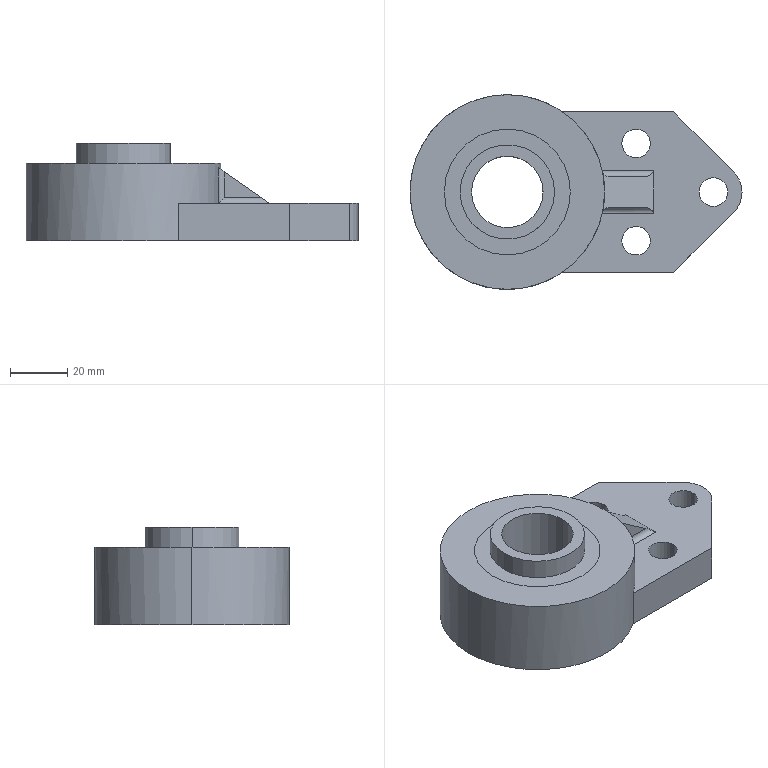Part | STEP file | UCFB205_1 | 2 solids | 38 faces | box 116 x 68 x 34 mm | volume 110392 mm3 | cylinder 24 | plane 14 | commonest cylinder face diameters 10 x6 4 x4 33 x4 44 x4 20 x2 25 x2